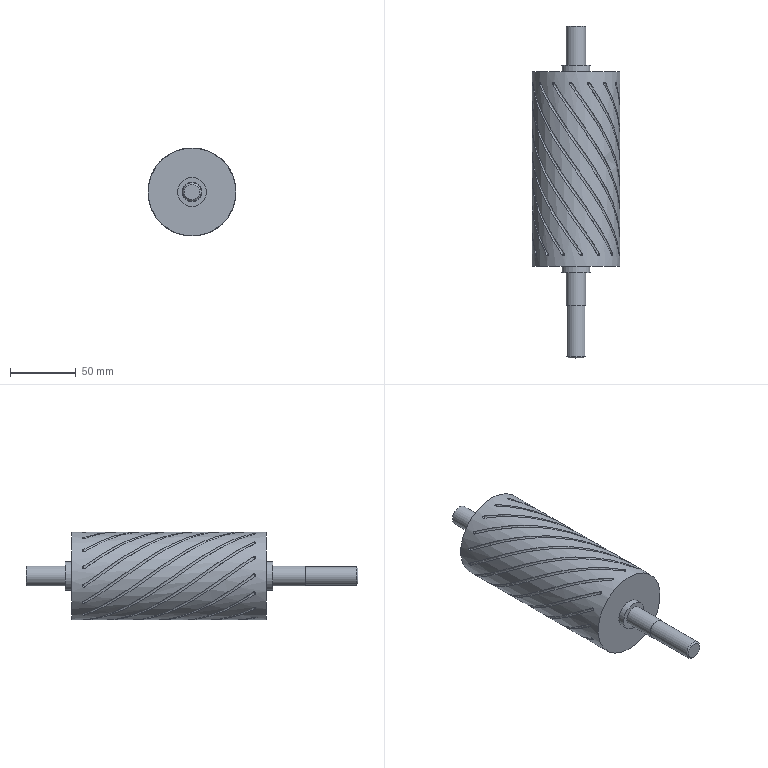Part | STEP file | YBQDJ-PD-9 | 1 solid | 89 faces | box 68.992 x 253 x 68.953 mm | volume 537694 mm3 | spline 45 | plane 37 | cylinder 6 | cone 1 | commonest cylinder face diameters 15 x2 22 x2 14 x1 67 x1